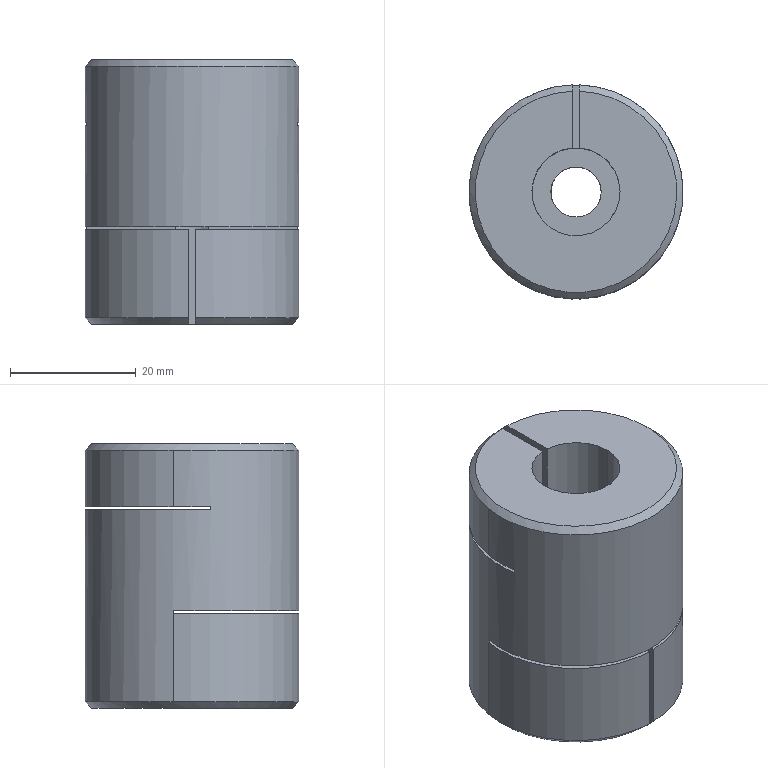Part | NX | 1 solid | 26 faces | box 34 x 34 x 42 mm | volume 33024 mm3 | plane 17 | cylinder 7 | cone 2 | commonest cylinder face diameters 34 x3 8 x2 14 x2
STEP:
#1=CARTESIAN_POINT('',(0.5,-3.969,-6.));
#2=VERTEX_POINT('',#1);
#3=CARTESIAN_POINT('',(2.646,3.,-6.));
#4=VERTEX_POINT('',#3);
#5=CARTESIAN_POINT('',(0.,0.,-6.));
#6=DIRECTION('',(0.,0.,-1.));
#7=DIRECTION('',(-1.,0.,0.));
#8=AXIS2_PLACEMENT_3D('',#5,#6,#7);
#9=CIRCLE('',#8,4.);
#10=EDGE_CURVE('',#2,#4,#9,.F.);
#11=ORIENTED_EDGE('',*,*,#10,.F.);
#12=CARTESIAN_POINT('',(0.5,-16.993,-6.));
#13=VERTEX_POINT('',#12);
#14=CARTESIAN_POINT('',(0.5,-17.,-6.));
#15=DIRECTION('',(0.,-1.,0.));
#16=VECTOR('',#15,1000.);
#17=LINE('',#14,#16);
#18=EDGE_CURVE('',#2,#13,#17,.T.);
#19=ORIENTED_EDGE('',*,*,#18,.T.);
#20=CARTESIAN_POINT('',(16.733,3.,-6.));
#21=VERTEX_POINT('',#20);
#22=CARTESIAN_POINT('',(0.,0.,-6.));
#23=DIRECTION('',(0.,0.,-1.));
#24=DIRECTION('',(-1.,0.,0.));
#25=AXIS2_PLACEMENT_3D('',#22,#23,#24);
#26=CIRCLE('',#25,17.);
#27=EDGE_CURVE('',#21,#13,#26,.T.);
#28=ORIENTED_EDGE('',*,*,#27,.F.);
#29=CARTESIAN_POINT('',(-22.75,3.,-6.));
#30=DIRECTION('',(1.,0.,0.));
#31=VECTOR('',#30,1000.);
#32=LINE('',#29,#31);
#33=EDGE_CURVE('',#4,#21,#32,.T.);
#34=ORIENTED_EDGE('',*,*,#33,.F.);
#35=EDGE_LOOP('',(#11,#19,#28,#34));
#36=FACE_BOUND('',#35,.T.);
#37=CARTESIAN_POINT('',(-22.75,-17.,-6.));
#38=DIRECTION('',(0.,0.,-1.));
#39=DIRECTION('',(-1.,0.,0.));
#40=AXIS2_PLACEMENT_3D('',#37,#38,#39);
#41=PLANE('',#40);
#42=ADVANCED_FACE('',(#36),#41,.F.);
#43=CARTESIAN_POINT('',(0.5,6.982,11.));
#44=VERTEX_POINT('',#43);
#45=CARTESIAN_POINT('',(6.325,-3.,11.));
#46=VERTEX_POINT('',#45);
#47=CARTESIAN_POINT('',(0.,0.,11.));
#48=DIRECTION('',(0.,0.,1.));
#49=DIRECTION('',(1.,0.,0.));
#50=AXIS2_PLACEMENT_3D('',#47,#48,#49);
#51=CIRCLE('',#50,7.);
#52=EDGE_CURVE('',#44,#46,#51,.F.);
#53=ORIENTED_EDGE('',*,*,#52,.F.);
#54=CARTESIAN_POINT('',(0.5,16.993,11.));
#55=VERTEX_POINT('',#54);
#56=CARTESIAN_POINT('',(0.5,17.,11.));
#57=DIRECTION('',(0.,1.,0.));
#58=VECTOR('',#57,1000.);
#59=LINE('',#56,#58);
#60=EDGE_CURVE('',#44,#55,#59,.T.);
#61=ORIENTED_EDGE('',*,*,#60,.T.);
#62=CARTESIAN_POINT('',(16.733,-3.,11.));
#63=VERTEX_POINT('',#62);
#64=CARTESIAN_POINT('',(0.,0.,11.));
#65=DIRECTION('',(0.,0.,1.));
#66=DIRECTION('',(1.,0.,0.));
#67=AXIS2_PLACEMENT_3D('',#64,#65,#66);
#68=CIRCLE('',#67,17.);
#69=EDGE_CURVE('',#63,#55,#68,.T.);
#70=ORIENTED_EDGE('',*,*,#69,.F.);
#71=CARTESIAN_POINT('',(-22.75,-3.,11.));
#72=DIRECTION('',(1.,0.,0.));
#73=VECTOR('',#72,1000.);
#74=LINE('',#71,#73);
#75=EDGE_CURVE('',#46,#63,#74,.T.);
#76=ORIENTED_EDGE('',*,*,#75,.F.);
#77=EDGE_LOOP('',(#53,#61,#70,#76));
#78=FACE_BOUND('',#77,.T.);
#79=CARTESIAN_POINT('',(-22.75,17.,11.));
#80=DIRECTION('',(0.,0.,1.));
#81=DIRECTION('',(1.,0.,0.));
#82=AXIS2_PLACEMENT_3D('',#79,#80,#81);
#83=PLANE('',#82);
#84=ADVANCED_FACE('',(#78),#83,.F.);
#85=CARTESIAN_POINT('',(0.5,-3.969,-21.));
#86=VERTEX_POINT('',#85);
#87=CARTESIAN_POINT('',(-0.5,-3.969,-21.));
#88=VERTEX_POINT('',#87);
#89=CARTESIAN_POINT('',(0.,0.,-21.));
#90=DIRECTION('',(0.,0.,1.));
#91=DIRECTION('',(1.,0.,0.));
#92=AXIS2_PLACEMENT_3D('',#89,#90,#91);
#93=CIRCLE('',#92,4.);
#94=EDGE_CURVE('',#86,#88,#93,.T.);
#95=ORIENTED_EDGE('',*,*,#94,.F.);
#96=CARTESIAN_POINT('',(0.5,-3.969,-21.));
#97=DIRECTION('',(0.,0.,1.));
#98=VECTOR('',#97,1000.);
#99=LINE('',#96,#98);
#100=EDGE_CURVE('',#86,#2,#99,.T.);
#101=ORIENTED_EDGE('',*,*,#100,.T.);
#102=ORIENTED_EDGE('',*,*,#10,.T.);
#103=CARTESIAN_POINT('',(2.646,3.,-5.5));
#104=VERTEX_POINT('',#103);
#105=CARTESIAN_POINT('',(2.646,3.,-21.));
#106=DIRECTION('',(0.,0.,1.));
#107=VECTOR('',#106,1000.);
#108=LINE('',#105,#107);
#109=EDGE_CURVE('',#4,#104,#108,.T.);
#110=ORIENTED_EDGE('',*,*,#109,.T.);
#111=CARTESIAN_POINT('',(-2.646,3.,-5.5));
#112=VERTEX_POINT('',#111);
#113=CARTESIAN_POINT('',(0.,0.,-5.5));
#114=DIRECTION('',(0.,0.,1.));
#115=DIRECTION('',(1.,0.,0.));
#116=AXIS2_PLACEMENT_3D('',#113,#114,#115);
#117=CIRCLE('',#116,4.);
#118=EDGE_CURVE('',#104,#112,#117,.F.);
#119=ORIENTED_EDGE('',*,*,#118,.T.);
#120=CARTESIAN_POINT('',(-2.646,3.,-6.));
#121=VERTEX_POINT('',#120);
#122=CARTESIAN_POINT('',(-2.646,3.,-21.));
#123=DIRECTION('',(0.,0.,1.));
#124=VECTOR('',#123,1000.);
#125=LINE('',#122,#124);
#126=EDGE_CURVE('',#112,#121,#125,.F.);
#127=ORIENTED_EDGE('',*,*,#126,.T.);
#128=CARTESIAN_POINT('',(-0.5,-3.969,-6.));
#129=VERTEX_POINT('',#128);
#130=CARTESIAN_POINT('',(0.,0.,-6.));
#131=DIRECTION('',(0.,0.,-1.));
#132=DIRECTION('',(-1.,0.,0.));
#133=AXIS2_PLACEMENT_3D('',#130,#131,#132);
#134=CIRCLE('',#133,4.);
#135=EDGE_CURVE('',#121,#129,#134,.F.);
#136=ORIENTED_EDGE('',*,*,#135,.T.);
#137=CARTESIAN_POINT('',(-0.5,-3.969,-21.));
#138=DIRECTION('',(0.,0.,1.));
#139=VECTOR('',#138,1000.);
#140=LINE('',#137,#139);
#141=EDGE_CURVE('',#129,#88,#140,.F.);
#142=ORIENTED_EDGE('',*,*,#141,.T.);
#143=EDGE_LOOP('',(#95,#101,#102,#110,#119,#127,#136,#142));
#144=FACE_BOUND('',#143,.T.);
#145=CARTESIAN_POINT('',(4.,0.,0.5));
#146=VERTEX_POINT('',#145);
#147=CARTESIAN_POINT('',(0.,0.,0.5));
#148=DIRECTION('',(0.,0.,1.));
#149=DIRECTION('',(1.,0.,0.));
#150=AXIS2_PLACEMENT_3D('',#147,#148,#149);
#151=CIRCLE('',#150,4.);
#152=EDGE_CURVE('',#146,#146,#151,.F.);
#153=ORIENTED_EDGE('',*,*,#152,.F.);
#154=EDGE_LOOP('',(#153));
#155=FACE_BOUND('',#154,.T.);
#156=CARTESIAN_POINT('',(0.,0.,-21.));
#157=DIRECTION('',(0.,0.,1.));
#158=DIRECTION('',(1.,0.,0.));
#159=AXIS2_PLACEMENT_3D('',#156,#157,#158);
#160=CYLINDRICAL_SURFACE('',#159,4.);
#161=ADVANCED_FACE('',(#144,#155),#160,.F.);
#162=CARTESIAN_POINT('',(0.5,16.993,20.));
#163=VERTEX_POINT('',#162);
#164=CARTESIAN_POINT('',(0.5,16.993,21.));
#165=DIRECTION('',(0.,0.,-1.));
#166=VECTOR('',#165,1000.);
#167=LINE('',#164,#166);
#168=EDGE_CURVE('',#55,#163,#167,.F.);
#169=ORIENTED_EDGE('',*,*,#168,.T.);
#170=CARTESIAN_POINT('',(-0.5,16.993,20.));
#171=VERTEX_POINT('',#170);
#172=CARTESIAN_POINT('',(0.,0.,20.));
#173=DIRECTION('',(0.,0.,1.));
#174=DIRECTION('',(1.,0.,0.));
#175=AXIS2_PLACEMENT_3D('',#172,#173,#174);
#176=CIRCLE('',#175,17.);
#177=EDGE_CURVE('',#163,#171,#176,.F.);
#178=ORIENTED_EDGE('',*,*,#177,.T.);
#179=CARTESIAN_POINT('',(-0.5,16.993,11.));
#180=VERTEX_POINT('',#179);
#181=CARTESIAN_POINT('',(-0.5,16.993,21.));
#182=DIRECTION('',(0.,0.,-1.));
#183=VECTOR('',#182,1000.);
#184=LINE('',#181,#183);
#185=EDGE_CURVE('',#171,#180,#184,.T.);
#186=ORIENTED_EDGE('',*,*,#185,.T.);
#187=CARTESIAN_POINT('',(-16.733,-3.,11.));
#188=VERTEX_POINT('',#187);
#189=CARTESIAN_POINT('',(0.,0.,11.));
#190=DIRECTION('',(0.,0.,1.));
#191=DIRECTION('',(1.,0.,0.));
#192=AXIS2_PLACEMENT_3D('',#189,#190,#191);
#193=CIRCLE('',#192,17.);
#194=EDGE_CURVE('',#180,#188,#193,.T.);
#195=ORIENTED_EDGE('',*,*,#194,.T.);
#196=CARTESIAN_POINT('',(-16.733,-3.,10.5));
#197=VERTEX_POINT('',#196);
#198=CARTESIAN_POINT('',(-16.733,-3.,21.));
#199=DIRECTION('',(0.,0.,-1.));
#200=VECTOR('',#199,1000.);
#201=LINE('',#198,#200);
#202=EDGE_CURVE('',#188,#197,#201,.T.);
#203=ORIENTED_EDGE('',*,*,#202,.T.);
#204=CARTESIAN_POINT('',(16.733,-3.,10.5));
#205=VERTEX_POINT('',#204);
#206=CARTESIAN_POINT('',(0.,0.,10.5));
#207=DIRECTION('',(0.,0.,-1.));
#208=DIRECTION('',(-1.,0.,0.));
#209=AXIS2_PLACEMENT_3D('',#206,#207,#208);
#210=CIRCLE('',#209,17.);
#211=EDGE_CURVE('',#197,#205,#210,.T.);
#212=ORIENTED_EDGE('',*,*,#211,.T.);
#213=CARTESIAN_POINT('',(16.733,-3.,21.));
#214=DIRECTION('',(0.,0.,-1.));
#215=VECTOR('',#214,1000.);
#216=LINE('',#213,#215);
#217=EDGE_CURVE('',#205,#63,#216,.F.);
#218=ORIENTED_EDGE('',*,*,#217,.T.);
#219=ORIENTED_EDGE('',*,*,#69,.T.);
#220=EDGE_LOOP('',(#169,#178,#186,#195,#203,#212,#218,#219));
#221=FACE_BOUND('',#220,.T.);
#222=CARTESIAN_POINT('',(0.5,-16.993,-20.));
#223=VERTEX_POINT('',#222);
#224=CARTESIAN_POINT('',(0.5,-16.993,21.));
#225=DIRECTION('',(0.,0.,-1.));
#226=VECTOR('',#225,1000.);
#227=LINE('',#224,#226);
#228=EDGE_CURVE('',#13,#223,#227,.T.);
#229=ORIENTED_EDGE('',*,*,#228,.T.);
#230=CARTESIAN_POINT('',(-0.5,-16.993,-20.));
#231=VERTEX_POINT('',#230);
#232=CARTESIAN_POINT('',(0.,0.,-20.));
#233=DIRECTION('',(0.,0.,1.));
#234=DIRECTION('',(1.,0.,0.));
#235=AXIS2_PLACEMENT_3D('',#232,#233,#234);
#236=CIRCLE('',#235,17.);
#237=EDGE_CURVE('',#223,#231,#236,.T.);
#238=ORIENTED_EDGE('',*,*,#237,.T.);
#239=CARTESIAN_POINT('',(-0.5,-16.993,-6.));
#240=VERTEX_POINT('',#239);
#241=CARTESIAN_POINT('',(-0.5,-16.993,21.));
#242=DIRECTION('',(0.,0.,-1.));
#243=VECTOR('',#242,1000.);
#244=LINE('',#241,#243);
#245=EDGE_CURVE('',#231,#240,#244,.F.);
#246=ORIENTED_EDGE('',*,*,#245,.T.);
#247=CARTESIAN_POINT('',(-16.733,3.,-6.));
#248=VERTEX_POINT('',#247);
#249=CARTESIAN_POINT('',(0.,0.,-6.));
#250=DIRECTION('',(0.,0.,-1.));
#251=DIRECTION('',(-1.,0.,0.));
#252=AXIS2_PLACEMENT_3D('',#249,#250,#251);
#253=CIRCLE('',#252,17.);
#254=EDGE_CURVE('',#240,#248,#253,.T.);
#255=ORIENTED_EDGE('',*,*,#254,.T.);
#256=CARTESIAN_POINT('',(-16.733,3.,-5.5));
#257=VERTEX_POINT('',#256);
#258=CARTESIAN_POINT('',(-16.733,3.,21.));
#259=DIRECTION('',(0.,0.,-1.));
#260=VECTOR('',#259,1000.);
#261=LINE('',#258,#260);
#262=EDGE_CURVE('',#248,#257,#261,.F.);
#263=ORIENTED_EDGE('',*,*,#262,.T.);
#264=CARTESIAN_POINT('',(16.733,3.,-5.5));
#265=VERTEX_POINT('',#264);
#266=CARTESIAN_POINT('',(0.,0.,-5.5));
#267=DIRECTION('',(0.,0.,1.));
#268=DIRECTION('',(1.,0.,0.));
#269=AXIS2_PLACEMENT_3D('',#266,#267,#268);
#270=CIRCLE('',#269,17.);
#271=EDGE_CURVE('',#257,#265,#270,.T.);
#272=ORIENTED_EDGE('',*,*,#271,.T.);
#273=CARTESIAN_POINT('',(16.733,3.,21.));
#274=DIRECTION('',(0.,0.,-1.));
#275=VECTOR('',#274,1000.);
#276=LINE('',#273,#275);
#277=EDGE_CURVE('',#265,#21,#276,.T.);
#278=ORIENTED_EDGE('',*,*,#277,.T.);
#279=ORIENTED_EDGE('',*,*,#27,.T.);
#280=EDGE_LOOP('',(#229,#238,#246,#255,#263,#272,#278,#279));
#281=FACE_BOUND('',#280,.T.);
#282=CARTESIAN_POINT('',(0.,0.,21.));
#283=DIRECTION('',(0.,0.,-1.));
#284=DIRECTION('',(-1.,0.,0.));
#285=AXIS2_PLACEMENT_3D('',#282,#283,#284);
#286=CYLINDRICAL_SURFACE('',#285,17.);
#287=ADVANCED_FACE('',(#221,#281),#286,.T.);
#288=CARTESIAN_POINT('',(-0.5,15.992,21.));
#289=VERTEX_POINT('',#288);
#290=CARTESIAN_POINT('',(-0.5,6.982,21.));
#291=VERTEX_POINT('',#290);
#292=CARTESIAN_POINT('',(-0.5,20.,21.));
#293=DIRECTION('',(0.,-1.,0.));
#294=VECTOR('',#293,1000.);
#295=LINE('',#292,#294);
#296=EDGE_CURVE('',#289,#291,#295,.T.);
#297=ORIENTED_EDGE('',*,*,#296,.F.);
#298=CARTESIAN_POINT('',(0.5,15.992,21.));
#299=VERTEX_POINT('',#298);
#300=CARTESIAN_POINT('',(0.,0.,21.));
#301=DIRECTION('',(0.,0.,1.));
#302=DIRECTION('',(1.,0.,0.));
#303=AXIS2_PLACEMENT_3D('',#300,#301,#302);
#304=CIRCLE('',#303,16.);
#305=EDGE_CURVE('',#289,#299,#304,.T.);
#306=ORIENTED_EDGE('',*,*,#305,.T.);
#307=CARTESIAN_POINT('',(0.5,6.982,21.));
#308=VERTEX_POINT('',#307);
#309=CARTESIAN_POINT('',(0.5,20.,21.));
#310=DIRECTION('',(0.,1.,0.));
#311=VECTOR('',#310,1000.);
#312=LINE('',#309,#311);
#313=EDGE_CURVE('',#308,#299,#312,.T.);
#314=ORIENTED_EDGE('',*,*,#313,.F.);
#315=CARTESIAN_POINT('',(0.,0.,21.));
#316=DIRECTION('',(0.,0.,1.));
#317=DIRECTION('',(1.,0.,0.));
#318=AXIS2_PLACEMENT_3D('',#315,#316,#317);
#319=CIRCLE('',#318,7.);
#320=EDGE_CURVE('',#291,#308,#319,.T.);
#321=ORIENTED_EDGE('',*,*,#320,.F.);
#322=EDGE_LOOP('',(#297,#306,#314,#321));
#323=FACE_BOUND('',#322,.T.);
#324=CARTESIAN_POINT('',(0.,0.,21.));
#325=DIRECTION('',(0.,0.,1.));
#326=DIRECTION('',(1.,0.,0.));
#327=AXIS2_PLACEMENT_3D('',#324,#325,#326);
#328=PLANE('',#327);
#329=ADVANCED_FACE('',(#323),#328,.T.);
#330=CARTESIAN_POINT('',(-0.5,-15.992,-21.));
#331=VERTEX_POINT('',#330);
#332=CARTESIAN_POINT('',(-0.5,0.,-21.));
#333=DIRECTION('',(0.,1.,0.));
#334=VECTOR('',#333,1000.);
#335=LINE('',#332,#334);
#336=EDGE_CURVE('',#331,#88,#335,.T.);
#337=ORIENTED_EDGE('',*,*,#336,.F.);
#338=CARTESIAN_POINT('',(0.5,-15.992,-21.));
#339=VERTEX_POINT('',#338);
#340=CARTESIAN_POINT('',(0.,0.,-21.));
#341=DIRECTION('',(0.,0.,1.));
#342=DIRECTION('',(1.,0.,0.));
#343=AXIS2_PLACEMENT_3D('',#340,#341,#342);
#344=CIRCLE('',#343,16.);
#345=EDGE_CURVE('',#331,#339,#344,.F.);
#346=ORIENTED_EDGE('',*,*,#345,.T.);
#347=CARTESIAN_POINT('',(0.5,0.,-21.));
#348=DIRECTION('',(0.,-1.,0.));
#349=VECTOR('',#348,1000.);
#350=LINE('',#347,#349);
#351=EDGE_CURVE('',#86,#339,#350,.T.);
#352=ORIENTED_EDGE('',*,*,#351,.F.);
#353=ORIENTED_EDGE('',*,*,#94,.T.);
#354=EDGE_LOOP('',(#337,#346,#352,#353));
#355=FACE_BOUND('',#354,.T.);
#356=CARTESIAN_POINT('',(0.,0.,-21.));
#357=DIRECTION('',(0.,0.,1.));
#358=DIRECTION('',(1.,0.,0.));
#359=AXIS2_PLACEMENT_3D('',#356,#357,#358);
#360=PLANE('',#359);
#361=ADVANCED_FACE('',(#355),#360,.F.);
#362=CARTESIAN_POINT('',(7.,0.,0.5));
#363=VERTEX_POINT('',#362);
#364=CARTESIAN_POINT('',(0.,0.,0.5));
#365=DIRECTION('',(0.,0.,1.));
#366=DIRECTION('',(1.,0.,0.));
#367=AXIS2_PLACEMENT_3D('',#364,#365,#366);
#368=CIRCLE('',#367,7.);
#369=EDGE_CURVE('',#363,#363,#368,.T.);
#370=ORIENTED_EDGE('',*,*,#369,.T.);
#371=EDGE_LOOP('',(#370));
#372=FACE_BOUND('',#371,.T.);
#373=ORIENTED_EDGE('',*,*,#152,.T.);
#374=EDGE_LOOP('',(#373));
#375=FACE_BOUND('',#374,.T.);
#376=CARTESIAN_POINT('',(0.,0.,0.5));
#377=DIRECTION('',(0.,0.,1.));
#378=DIRECTION('',(1.,0.,0.));
#379=AXIS2_PLACEMENT_3D('',#376,#377,#378);
#380=PLANE('',#379);
#381=ADVANCED_FACE('',(#372,#375),#380,.T.);
#382=ORIENTED_EDGE('',*,*,#320,.T.);
#383=CARTESIAN_POINT('',(0.5,6.982,0.5));
#384=DIRECTION('',(0.,0.,1.));
#385=VECTOR('',#384,1000.);
#386=LINE('',#383,#385);
#387=EDGE_CURVE('',#308,#44,#386,.F.);
#388=ORIENTED_EDGE('',*,*,#387,.T.);
#389=ORIENTED_EDGE('',*,*,#52,.T.);
#390=CARTESIAN_POINT('',(6.325,-3.,10.5));
#391=VERTEX_POINT('',#390);
#392=CARTESIAN_POINT('',(6.325,-3.,0.5));
#393=DIRECTION('',(0.,0.,1.));
#394=VECTOR('',#393,1000.);
#395=LINE('',#392,#394);
#396=EDGE_CURVE('',#46,#391,#395,.F.);
#397=ORIENTED_EDGE('',*,*,#396,.T.);
#398=CARTESIAN_POINT('',(-6.325,-3.,10.5));
#399=VERTEX_POINT('',#398);
#400=CARTESIAN_POINT('',(0.,0.,10.5));
#401=DIRECTION('',(0.,0.,-1.));
#402=DIRECTION('',(-1.,0.,0.));
#403=AXIS2_PLACEMENT_3D('',#400,#401,#402);
#404=CIRCLE('',#403,7.);
#405=EDGE_CURVE('',#391,#399,#404,.F.);
#406=ORIENTED_EDGE('',*,*,#405,.T.);
#407=CARTESIAN_POINT('',(-6.325,-3.,11.));
#408=VERTEX_POINT('',#407);
#409=CARTESIAN_POINT('',(-6.325,-3.,0.5));
#410=DIRECTION('',(0.,0.,1.));
#411=VECTOR('',#410,1000.);
#412=LINE('',#409,#411);
#413=EDGE_CURVE('',#399,#408,#412,.T.);
#414=ORIENTED_EDGE('',*,*,#413,.T.);
#415=CARTESIAN_POINT('',(-0.5,6.982,11.));
#416=VERTEX_POINT('',#415);
#417=CARTESIAN_POINT('',(0.,0.,11.));
#418=DIRECTION('',(0.,0.,1.));
#419=DIRECTION('',(1.,0.,0.));
#420=AXIS2_PLACEMENT_3D('',#417,#418,#419);
#421=CIRCLE('',#420,7.);
#422=EDGE_CURVE('',#408,#416,#421,.F.);
#423=ORIENTED_EDGE('',*,*,#422,.T.);
#424=CARTESIAN_POINT('',(-0.5,6.982,0.5));
#425=DIRECTION('',(0.,0.,1.));
#426=VECTOR('',#425,1000.);
#427=LINE('',#424,#426);
#428=EDGE_CURVE('',#416,#291,#427,.T.);
#429=ORIENTED_EDGE('',*,*,#428,.T.);
#430=EDGE_LOOP('',(#382,#388,#389,#397,#406,#414,#423,#429));
#431=FACE_BOUND('',#430,.T.);
#432=ORIENTED_EDGE('',*,*,#369,.F.);
#433=EDGE_LOOP('',(#432));
#434=FACE_BOUND('',#433,.T.);
#435=CARTESIAN_POINT('',(0.,0.,0.5));
#436=DIRECTION('',(0.,0.,1.));
#437=DIRECTION('',(1.,0.,0.));
#438=AXIS2_PLACEMENT_3D('',#435,#436,#437);
#439=CYLINDRICAL_SURFACE('',#438,7.);
#440=ADVANCED_FACE('',(#431,#434),#439,.F.);
#441=ORIENTED_EDGE('',*,*,#194,.F.);
#442=CARTESIAN_POINT('',(-0.5,17.,11.));
#443=DIRECTION('',(0.,-1.,0.));
#444=VECTOR('',#443,1000.);
#445=LINE('',#442,#444);
#446=EDGE_CURVE('',#180,#416,#445,.T.);
#447=ORIENTED_EDGE('',*,*,#446,.T.);
#448=ORIENTED_EDGE('',*,*,#422,.F.);
#449=CARTESIAN_POINT('',(-22.75,-3.,11.));
#450=DIRECTION('',(1.,0.,0.));
#451=VECTOR('',#450,1000.);
#452=LINE('',#449,#451);
#453=EDGE_CURVE('',#188,#408,#452,.T.);
#454=ORIENTED_EDGE('',*,*,#453,.F.);
#455=EDGE_LOOP('',(#441,#447,#448,#454));
#456=FACE_BOUND('',#455,.T.);
#457=CARTESIAN_POINT('',(-22.75,17.,11.));
#458=DIRECTION('',(0.,0.,1.));
#459=DIRECTION('',(1.,0.,0.));
#460=AXIS2_PLACEMENT_3D('',#457,#458,#459);
#461=PLANE('',#460);
#462=ADVANCED_FACE('',(#456),#461,.F.);
#463=CARTESIAN_POINT('',(-22.75,-3.,10.5));
#464=DIRECTION('',(1.,0.,0.));
#465=VECTOR('',#464,1000.);
#466=LINE('',#463,#465);
#467=EDGE_CURVE('',#197,#399,#466,.T.);
#468=ORIENTED_EDGE('',*,*,#467,.T.);
#469=ORIENTED_EDGE('',*,*,#405,.F.);
#470=CARTESIAN_POINT('',(-22.75,-3.,10.5));
#471=DIRECTION('',(1.,0.,0.));
#472=VECTOR('',#471,1000.);
#473=LINE('',#470,#472);
#474=EDGE_CURVE('',#391,#205,#473,.T.);
#475=ORIENTED_EDGE('',*,*,#474,.T.);
#476=ORIENTED_EDGE('',*,*,#211,.F.);
#477=EDGE_LOOP('',(#468,#469,#475,#476));
#478=FACE_BOUND('',#477,.T.);
#479=CARTESIAN_POINT('',(-22.75,17.,10.5));
#480=DIRECTION('',(0.,0.,-1.));
#481=DIRECTION('',(-1.,0.,0.));
#482=AXIS2_PLACEMENT_3D('',#479,#480,#481);
#483=PLANE('',#482);
#484=ADVANCED_FACE('',(#478),#483,.F.);
#485=ORIENTED_EDGE('',*,*,#453,.T.);
#486=ORIENTED_EDGE('',*,*,#413,.F.);
#487=ORIENTED_EDGE('',*,*,#467,.F.);
#488=ORIENTED_EDGE('',*,*,#202,.F.);
#489=EDGE_LOOP('',(#485,#486,#487,#488));
#490=FACE_BOUND('',#489,.T.);
#491=CARTESIAN_POINT('',(-22.75,-3.,11.));
#492=DIRECTION('',(0.,-1.,0.));
#493=DIRECTION('',(0.,0.,-1.));
#494=AXIS2_PLACEMENT_3D('',#491,#492,#493);
#495=PLANE('',#494);
#496=ADVANCED_FACE('',(#490),#495,.F.);
#497=ORIENTED_EDGE('',*,*,#474,.F.);
#498=ORIENTED_EDGE('',*,*,#396,.F.);
#499=ORIENTED_EDGE('',*,*,#75,.T.);
#500=ORIENTED_EDGE('',*,*,#217,.F.);
#501=EDGE_LOOP('',(#497,#498,#499,#500));
#502=FACE_BOUND('',#501,.T.);
#503=CARTESIAN_POINT('',(-22.75,-3.,11.));
#504=DIRECTION('',(0.,-1.,0.));
#505=DIRECTION('',(0.,0.,-1.));
#506=AXIS2_PLACEMENT_3D('',#503,#504,#505);
#507=PLANE('',#506);
#508=ADVANCED_FACE('',(#502),#507,.F.);
#509=ORIENTED_EDGE('',*,*,#254,.F.);
#510=CARTESIAN_POINT('',(-0.5,-17.,-6.));
#511=DIRECTION('',(0.,1.,0.));
#512=VECTOR('',#511,1000.);
#513=LINE('',#510,#512);
#514=EDGE_CURVE('',#240,#129,#513,.T.);
#515=ORIENTED_EDGE('',*,*,#514,.T.);
#516=ORIENTED_EDGE('',*,*,#135,.F.);
#517=CARTESIAN_POINT('',(-22.75,3.,-6.));
#518=DIRECTION('',(1.,0.,0.));
#519=VECTOR('',#518,1000.);
#520=LINE('',#517,#519);
#521=EDGE_CURVE('',#248,#121,#520,.T.);
#522=ORIENTED_EDGE('',*,*,#521,.F.);
#523=EDGE_LOOP('',(#509,#515,#516,#522));
#524=FACE_BOUND('',#523,.T.);
#525=CARTESIAN_POINT('',(-22.75,-17.,-6.));
#526=DIRECTION('',(0.,0.,-1.));
#527=DIRECTION('',(-1.,0.,0.));
#528=AXIS2_PLACEMENT_3D('',#525,#526,#527);
#529=PLANE('',#528);
#530=ADVANCED_FACE('',(#524),#529,.F.);
#531=CARTESIAN_POINT('',(-22.75,3.,-5.5));
#532=DIRECTION('',(1.,0.,0.));
#533=VECTOR('',#532,1000.);
#534=LINE('',#531,#533);
#535=EDGE_CURVE('',#257,#112,#534,.T.);
#536=ORIENTED_EDGE('',*,*,#535,.T.);
#537=ORIENTED_EDGE('',*,*,#118,.F.);
#538=CARTESIAN_POINT('',(-22.75,3.,-5.5));
#539=DIRECTION('',(1.,0.,0.));
#540=VECTOR('',#539,1000.);
#541=LINE('',#538,#540);
#542=EDGE_CURVE('',#104,#265,#541,.T.);
#543=ORIENTED_EDGE('',*,*,#542,.T.);
#544=ORIENTED_EDGE('',*,*,#271,.F.);
#545=EDGE_LOOP('',(#536,#537,#543,#544));
#546=FACE_BOUND('',#545,.T.);
#547=CARTESIAN_POINT('',(-22.75,-17.,-5.5));
#548=DIRECTION('',(0.,0.,1.));
#549=DIRECTION('',(1.,0.,0.));
#550=AXIS2_PLACEMENT_3D('',#547,#548,#549);
#551=PLANE('',#550);
#552=ADVANCED_FACE('',(#546),#551,.F.);
#553=ORIENTED_EDGE('',*,*,#535,.F.);
#554=ORIENTED_EDGE('',*,*,#262,.F.);
#555=ORIENTED_EDGE('',*,*,#521,.T.);
#556=ORIENTED_EDGE('',*,*,#126,.F.);
#557=EDGE_LOOP('',(#553,#554,#555,#556));
#558=FACE_BOUND('',#557,.T.);
#559=CARTESIAN_POINT('',(-22.75,3.,-6.));
#560=DIRECTION('',(0.,1.,0.));
#561=DIRECTION('',(0.,0.,1.));
#562=AXIS2_PLACEMENT_3D('',#559,#560,#561);
#563=PLANE('',#562);
#564=ADVANCED_FACE('',(#558),#563,.F.);
#565=ORIENTED_EDGE('',*,*,#33,.T.);
#566=ORIENTED_EDGE('',*,*,#277,.F.);
#567=ORIENTED_EDGE('',*,*,#542,.F.);
#568=ORIENTED_EDGE('',*,*,#109,.F.);
#569=EDGE_LOOP('',(#565,#566,#567,#568));
#570=FACE_BOUND('',#569,.T.);
#571=CARTESIAN_POINT('',(-22.75,3.,-6.));
#572=DIRECTION('',(0.,1.,0.));
#573=DIRECTION('',(0.,0.,1.));
#574=AXIS2_PLACEMENT_3D('',#571,#572,#573);
#575=PLANE('',#574);
#576=ADVANCED_FACE('',(#570),#575,.F.);
#577=ORIENTED_EDGE('',*,*,#185,.F.);
#578=CARTESIAN_POINT('',(-0.5,16.993,20.));
#579=CARTESIAN_POINT('',(-0.5,16.659,20.333));
#580=CARTESIAN_POINT('',(-0.5,16.326,20.667));
#581=CARTESIAN_POINT('',(-0.5,15.992,21.));
#582=B_SPLINE_CURVE_WITH_KNOTS('',3,(#578,#579,#580,#581),.UNSPECIFIED.,.F.,.F.,(4,4),(0.,0.001415),.UNSPECIFIED.);
#583=EDGE_CURVE('',#171,#289,#582,.T.);
#584=ORIENTED_EDGE('',*,*,#583,.T.);
#585=ORIENTED_EDGE('',*,*,#296,.T.);
#586=ORIENTED_EDGE('',*,*,#428,.F.);
#587=ORIENTED_EDGE('',*,*,#446,.F.);
#588=EDGE_LOOP('',(#577,#584,#585,#586,#587));
#589=FACE_BOUND('',#588,.T.);
#590=CARTESIAN_POINT('',(-0.5,20.,-9.525));
#591=DIRECTION('',(-1.,0.,0.));
#592=DIRECTION('',(0.,-1.,0.));
#593=AXIS2_PLACEMENT_3D('',#590,#591,#592);
#594=PLANE('',#593);
#595=ADVANCED_FACE('',(#589),#594,.F.);
#596=ORIENTED_EDGE('',*,*,#313,.T.);
#597=CARTESIAN_POINT('',(0.5,15.992,21.));
#598=CARTESIAN_POINT('',(0.5,16.326,20.667));
#599=CARTESIAN_POINT('',(0.5,16.659,20.333));
#600=CARTESIAN_POINT('',(0.5,16.993,20.));
#601=B_SPLINE_CURVE_WITH_KNOTS('',3,(#597,#598,#599,#600),.UNSPECIFIED.,.F.,.F.,(4,4),(0.,0.001415),.UNSPECIFIED.);
#602=EDGE_CURVE('',#299,#163,#601,.T.);
#603=ORIENTED_EDGE('',*,*,#602,.T.);
#604=ORIENTED_EDGE('',*,*,#168,.F.);
#605=ORIENTED_EDGE('',*,*,#60,.F.);
#606=ORIENTED_EDGE('',*,*,#387,.F.);
#607=EDGE_LOOP('',(#596,#603,#604,#605,#606));
#608=FACE_BOUND('',#607,.T.);
#609=CARTESIAN_POINT('',(0.5,20.,-9.525));
#610=DIRECTION('',(1.,0.,0.));
#611=DIRECTION('',(0.,1.,0.));
#612=AXIS2_PLACEMENT_3D('',#609,#610,#611);
#613=PLANE('',#612);
#614=ADVANCED_FACE('',(#608),#613,.F.);
#615=ORIENTED_EDGE('',*,*,#245,.F.);
#616=CARTESIAN_POINT('',(-0.5,-16.993,-20.));
#617=CARTESIAN_POINT('',(-0.5,-16.659,-20.333));
#618=CARTESIAN_POINT('',(-0.5,-16.326,-20.667));
#619=CARTESIAN_POINT('',(-0.5,-15.992,-21.));
#620=B_SPLINE_CURVE_WITH_KNOTS('',3,(#616,#617,#618,#619),.UNSPECIFIED.,.F.,.F.,(4,4),(0.,0.001415),.UNSPECIFIED.);
#621=EDGE_CURVE('',#231,#331,#620,.T.);
#622=ORIENTED_EDGE('',*,*,#621,.T.);
#623=ORIENTED_EDGE('',*,*,#336,.T.);
#624=ORIENTED_EDGE('',*,*,#141,.F.);
#625=ORIENTED_EDGE('',*,*,#514,.F.);
#626=EDGE_LOOP('',(#615,#622,#623,#624,#625));
#627=FACE_BOUND('',#626,.T.);
#628=CARTESIAN_POINT('',(-0.5,0.,19.52));
#629=DIRECTION('',(-1.,0.,0.));
#630=DIRECTION('',(0.,-1.,0.));
#631=AXIS2_PLACEMENT_3D('',#628,#629,#630);
#632=PLANE('',#631);
#633=ADVANCED_FACE('',(#627),#632,.F.);
#634=ORIENTED_EDGE('',*,*,#351,.T.);
#635=CARTESIAN_POINT('',(0.5,-15.992,-21.));
#636=CARTESIAN_POINT('',(0.5,-16.326,-20.667));
#637=CARTESIAN_POINT('',(0.5,-16.659,-20.333));
#638=CARTESIAN_POINT('',(0.5,-16.993,-20.));
#639=B_SPLINE_CURVE_WITH_KNOTS('',3,(#635,#636,#637,#638),.UNSPECIFIED.,.F.,.F.,(4,4),(0.,0.001415),.UNSPECIFIED.);
#640=EDGE_CURVE('',#339,#223,#639,.T.);
#641=ORIENTED_EDGE('',*,*,#640,.T.);
#642=ORIENTED_EDGE('',*,*,#228,.F.);
#643=ORIENTED_EDGE('',*,*,#18,.F.);
#644=ORIENTED_EDGE('',*,*,#100,.F.);
#645=EDGE_LOOP('',(#634,#641,#642,#643,#644));
#646=FACE_BOUND('',#645,.T.);
#647=CARTESIAN_POINT('',(0.5,0.,19.52));
#648=DIRECTION('',(1.,0.,0.));
#649=DIRECTION('',(0.,1.,0.));
#650=AXIS2_PLACEMENT_3D('',#647,#648,#649);
#651=PLANE('',#650);
#652=ADVANCED_FACE('',(#646),#651,.F.);
#653=ORIENTED_EDGE('',*,*,#583,.F.);
#654=ORIENTED_EDGE('',*,*,#177,.F.);
#655=ORIENTED_EDGE('',*,*,#602,.F.);
#656=ORIENTED_EDGE('',*,*,#305,.F.);
#657=EDGE_LOOP('',(#653,#654,#655,#656));
#658=FACE_BOUND('',#657,.T.);
#659=CARTESIAN_POINT('',(0.,0.,21.));
#660=DIRECTION('',(0.,0.,-1.));
#661=DIRECTION('',(-1.,0.,0.));
#662=AXIS2_PLACEMENT_3D('',#659,#660,#661);
#663=CONICAL_SURFACE('',#662,16.,0.7854);
#664=ADVANCED_FACE('',(#658),#663,.T.);
#665=ORIENTED_EDGE('',*,*,#640,.F.);
#666=ORIENTED_EDGE('',*,*,#345,.F.);
#667=ORIENTED_EDGE('',*,*,#621,.F.);
#668=ORIENTED_EDGE('',*,*,#237,.F.);
#669=EDGE_LOOP('',(#665,#666,#667,#668));
#670=FACE_BOUND('',#669,.T.);
#671=CARTESIAN_POINT('',(0.,0.,-20.));
#672=DIRECTION('',(0.,0.,1.));
#673=DIRECTION('',(1.,0.,0.));
#674=AXIS2_PLACEMENT_3D('',#671,#672,#673);
#675=CONICAL_SURFACE('',#674,17.,0.7854);
#676=ADVANCED_FACE('',(#670),#675,.T.);
#677=CLOSED_SHELL('',(#42,#84,#161,#287,#329,#361,#381,#440,#462,#484,#496,#508,#530,#552,#564,#576,#595,#614,#633,#652,#664,#676));
#678=MANIFOLD_SOLID_BREP('',#677);
#679=(LENGTH_UNIT()NAMED_UNIT(*)SI_UNIT(.MILLI.,.METRE.));
#680=UNCERTAINTY_MEASURE_WITH_UNIT(LENGTH_MEASURE(0.0508),#679,'','');
#681=(NAMED_UNIT(*)PLANE_ANGLE_UNIT()SI_UNIT($,.RADIAN.));
#682=(NAMED_UNIT(*)SI_UNIT($,.STERADIAN.)SOLID_ANGLE_UNIT());
#683=(GEOMETRIC_REPRESENTATION_CONTEXT(3)GLOBAL_UNCERTAINTY_ASSIGNED_CONTEXT((#680))GLOBAL_UNIT_ASSIGNED_CONTEXT((#679,#681,#682))REPRESENTATION_CONTEXT('',''));
#684=ADVANCED_BREP_SHAPE_REPRESENTATION('',(#678),#683);